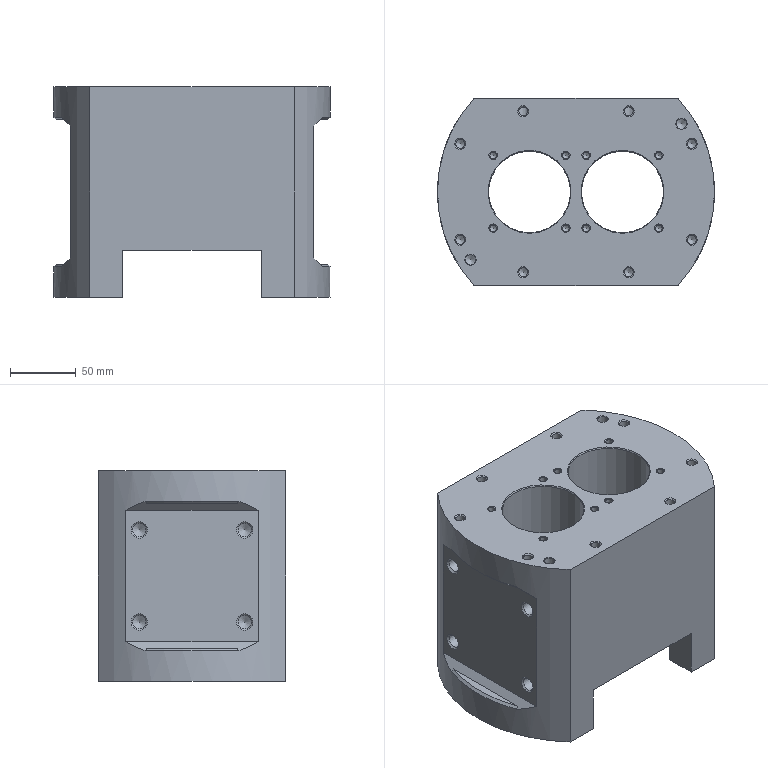NC program | NX | posted with a generic post | part box 210 x 142 x 160 mm
Lines 2120 to 2980 of 4730:
(ZLEVEL_PROFILE_COPY_1 , TOOL : D6R0.5)
N4226 T05 M6
N4228 G54
N4230 G17 G0 G90 X-53.624 Y12.862 B0. C0. S6500 M3
N4232 G43 Z30. H5
N4234 Z2.929
N4236 G94 G1 Z-0.071 F1000.
N4238 X-54.419 Y12.28
N4240 G3 X-54.662 Y11.731 R0.6
N4242 G2 X-54.662 Y-11.732 R108.942 F2500.
N4244 G1 X-54.661 Y-11.887 Z-0.088
N4246 Y-12.042 Z-0.106
N4248 X-54.662 Y-12.197 Z-0.124
N4250 X-54.665 Y-12.351 Z-0.141
N4252 G3 X-54.664 Y12.355 R108.184
N4254 G1 X-54.663 Y12.506 Z-0.159
N4256 Y12.656 Z-0.177
N4258 X-54.664 Y12.806 Z-0.194
N4260 X-54.667 Y12.956 Z-0.212
N4262 G2 X-54.667 Y-12.956 R107.566
N4264 G1 X-54.664 Y-13.103 Z-0.23
N4266 X-54.665 Y-13.25 Z-0.247
N4268 Y-13.397 Z-0.265
N4270 X-54.667 Y-13.544 Z-0.283
N4272 G3 X-54.667 Y13.542 R108.057
N4274 G1 X-54.666 Y13.687 Z-0.301
N4276 X-54.667 Y13.831 Z-0.318
N4278 Y13.976 Z-0.336
N4280 X-54.669 Y14.12 Z-0.354
N4282 G2 X-54.668 Y-14.125 R108.183
N4284 G1 X-54.666 Y-14.262 Z-0.371
N4286 Y-14.399 Z-0.389
N4288 X-54.667 Y-14.536 Z-0.407
N4290 X-54.671 Y-14.673 Z-0.424
N4292 G3 X-54.671 Y14.674 R108.33
N4294 G1 X-54.667 Y14.844 Z-0.448
N4296 X-54.668 Y15.013 Z-0.471
N4298 X-54.671 Y15.183 Z-0.495
N4300 G2 X-54.671 Y-15.18 R108.224
N4302 G1 Y-15.344 Z-0.519
N4304 Y-15.508 Z-0.542
N4306 X-54.674 Y-15.672 Z-0.566
N4308 G3 X-54.674 Y15.674 R107.882
N4310 G1 X-54.672 Y15.835 Z-0.589
N4312 Y15.997 Z-0.613
N4314 X-54.675 Y16.158 Z-0.636
N4316 G2 X-54.675 Y-16.159 R107.945
N4318 G1 X-54.673 Y-16.318 Z-0.66
N4320 X-54.674 Y-16.476 Z-0.684
N4322 X-54.675 Y-16.635 Z-0.707
N4324 G3 X-54.675 Y16.633 R108.072
N4326 G1 Y16.79 Z-0.731
N4328 Y16.946 Z-0.754
N4330 X-54.679 Y17.103 Z-0.778
N4332 G2 X-54.678 Y-17.107 R108.254
N4334 G1 X-54.675 Y-17.257 Z-0.801
N4336 X-54.676 Y-17.407 Z-0.825
N4338 X-54.679 Y-17.556 Z-0.849
N4340 G3 X-54.679 Y17.557 R108.475
N4342 G1 X-54.677 Y17.702 Z-0.872
N4344 Y17.846 Z-0.896
N4346 X-54.679 Y17.99 Z-0.919
N4348 G2 X-54.679 Y-17.988 R108.62
N4350 G1 X-54.68 Y-18.126 Z-0.943
N4352 Y-18.264 Z-0.966
N4354 X-54.682 Y-18.402 Z-0.99
N4356 G3 X-54.682 Y18.404 R108.324
N4358 G1 X-54.681 Y18.541 Z-1.014
N4360 Y18.678 Z-1.037
N4362 X-54.685 Y18.815 Z-1.061
N4364 G2 X-54.685 Y-18.815 R108.248
N4366 G1 X-54.682 Y-18.951 Z-1.084
N4368 X-54.683 Y-19.086 Z-1.108
N4370 X-54.686 Y-19.221 Z-1.131
N4372 G3 X-54.686 Y19.221 R108.276
N4374 G1 X-54.684 Y19.354 Z-1.155
N4376 X-54.685 Y19.487 Z-1.179
N4378 X-54.687 Y19.62 Z-1.202
N4380 G2 X-54.687 Y-19.622 R108.378
N4382 G1 X-54.685 Y-19.756 Z-1.226
N4384 Y-19.889 Z-1.249
N4386 X-54.687 Y-20.022 Z-1.273
N4388 G3 X-54.688 Y20.019 R108.63
N4390 G1 X-54.687 Y20.147 Z-1.296
N4392 Y20.274 Z-1.32
N4394 X-54.688 Y20.401 Z-1.344
N4396 G2 X-54.688 Y-20.401 R108.747
N4398 G1 Y-20.526 Z-1.367
N4400 Y-20.65 Z-1.391
N4402 X-54.69 Y-20.775 Z-1.414
N4404 G3 X-54.689 Y20.778 R108.773
N4406 G1 Y20.897 Z-1.438
N4408 X-54.69 Y21.016 Z-1.461
N4410 X-54.691 Y21.135 Z-1.485
N4412 G2 X-54.691 Y-21.132 R108.599
N4414 G1 Y-21.251 Z-1.508
N4416 X-54.692 Y-21.37 Z-1.532
N4418 X-54.693 Y-21.489 Z-1.556
N4420 G3 X-54.693 Y21.49 R108.585
N4422 G1 X-54.692 Y21.608 Z-1.579
N4424 X-54.693 Y21.726 Z-1.603
N4426 X-54.695 Y21.844 Z-1.626
N4428 G2 X-54.695 Y-21.844 R108.601
N4430 G1 X-54.694 Y-22.017 Z-1.662
N4432 X-54.695 Y-22.189 Z-1.697
N4434 G3 X-54.695 Y22.188 R108.586
N4436 G1 Y22.36 Z-1.732
N4438 X-54.696 Y22.531 Z-1.768
N4440 G2 X-52.49 Y-5.881 R108.93
N4442 X-54.696 Y-22.532 R111.727
N4444 G1 X-54.695 Y-22.703 Z-1.803
N4446 X-54.696 Y-22.874 Z-1.838
N4448 G3 X-52.291 Y-2.768 R111.416
N4450 X-54.697 Y22.872 R109.773
N4452 G1 X-54.696 Y23.036 Z-1.874
N4454 X-54.697 Y23.2 Z-1.909
N4456 G2 X-52.22 Y-2.768 R110.042
N4458 X-54.697 Y-23.2 R111.413
N4460 G1 Y-23.362 Z-1.945
N4462 X-54.698 Y-23.524 Z-1.98
N4464 G3 X-52.152 Y2.768 R109.879
N4466 X-54.697 Y23.525 R111.361
N4468 G1 X-54.696 Y23.683 Z-2.015
N4470 X-54.698 Y23.84 Z-2.051
N4472 G2 X-52.188 Y5.535 R112.247
N4474 X-52.188 Y-5.535 R122.471
N4476 X-54.699 Y-23.838 R112.088
N4478 G1 Y-23.992 Z-2.086
N4480 X-54.7 Y-24.146 Z-2.122
N4482 G3 X-52.121 Y-5.535 R111.188
N4484 X-52.121 Y5.535 R171.637
N4486 X-54.7 Y24.148 R111.301
N4488 G1 X-54.699 Y24.302 Z-2.157
N4490 X-54.702 Y24.454 Z-2.192
N4492 G2 X-52.227 Y8.302 R112.524
N4494 G1 X-52.084 Y5.881
N4496 X-52.07 Y5.535
N4498 G2 X-52.07 Y-5.535 R256.64
N4500 X-53.483 Y-18.335 R102.084
N4502 X-54.702 Y-24.454 R104.38
N4504 G1 X-54.7 Y-24.609 Z-2.228
N4506 X-54.703 Y-24.762 Z-2.263
N4508 G3 X-52.28 Y-9.779 R111.73
N4510 X-52.023 Y-4.713 R60.658
N4512 X-52.023 Y4.713 R498.143
N4514 X-52.159 Y8.302 R64.784
N4516 X-54.703 Y24.762 R111.682
N4518 G1 X-54.701 Y24.916 Z-2.299
N4520 X-54.704 Y25.069 Z-2.334
N4522 G2 X-52.097 Y8.302 R109.91
N4524 X-52. Y3.91 R99.303
N4526 G1 Y-3.91
N4528 G2 X-52.097 Y-8.302 R99.276
N4530 X-54.704 Y-25.071 R109.974
N4532 G1 X-54.702 Y-25.225 Z-2.37
N4534 X-54.705 Y-25.379 Z-2.405
N4536 G3 X-53.78 Y-21.102 R105.979
N4538 X-52.092 Y-8.994 R103.636
N4540 X-52. Y-5.554 R64.677
N4542 G1 Y4.497
N4544 G3 X-52.056 Y8.302 R101.781
N4546 X-52.268 Y11.07 R50.215
N4548 X-54.705 Y25.377 R113.821
N4550 G1 X-54.703 Y25.53 Z-2.441
N4552 X-54.706 Y25.682 Z-2.477
N4554 G2 X-52.203 Y11.127 R114.462
N4556 X-52.021 Y8.053 R33.214
N4558 G1 X-52.002 Y6.573
N4560 X-52.001 Y6.227
N4562 X-52. Y6.034
N4564 Y-6.043
N4566 X-52.002 Y-6.573
N4568 X-52.021 Y-8.033
N4570 G2 X-52.208 Y-11.166 R33.626
N4572 X-54.705 Y-25.684 R115.067
N4574 G1 X-54.704 Y-25.832 Z-2.512
N4576 X-54.706 Y-25.979 Z-2.548
N4578 G3 X-52.132 Y-11.07 R113.634
N4580 X-52. Y-7.145 R49.439
N4582 G1 Y7.148
N4584 G3 X-52.132 Y11.07 R49.422
N4586 X-54.706 Y25.978 R113.527
N4588 G1 Y26.125 Z-2.583
N4590 X-54.707 Y26.271 Z-2.619
N4592 G2 X-52.104 Y11.416 R111.997
N4594 X-52. Y8.105 R46.027
N4596 G1 Y-8.107
N4598 G2 X-52.104 Y-11.416 R46.02
N4600 X-54.707 Y-26.271 R111.928
N4602 G1 Y-26.415 Z-2.654
N4604 X-54.709 Y-26.56 Z-2.69
N4606 G3 X-52.31 Y-13.837 R115.903
N4608 G1 X-52.203 Y-12.938
N4610 G3 X-52. Y-9.511 R28.979
N4612 G1 Y9.511
N4614 G3 X-52.203 Y12.938 R28.98
N4616 G1 X-52.31 Y13.837
N4618 G3 X-54.709 Y26.562 R116.198
N4620 G1 X-54.708 Y26.702 Z-2.726
N4622 X-54.711 Y26.842 Z-2.761
N4624 G2 X-52.273 Y14.101 R116.39
N4626 X-52. Y10.008 R30.803
N4628 G1 Y-10.002
N4630 G2 X-52.274 Y-14.106 R30.884
N4632 X-54.711 Y-26.84 R116.146
N4634 G1 X-54.71 Y-26.979 Z-2.797
N4636 X-54.712 Y-27.117 Z-2.833
N4638 G3 X-52.279 Y-14.701 R116.024
N4640 X-52. Y-10.474 R29.016
N4642 G1 Y10.472
N4644 G3 X-52.171 Y13.837 R29.025
N4646 X-54.712 Y27.118 R114.844
N4648 G1 X-54.711 Y27.257 Z-2.868
N4650 X-54.713 Y27.395 Z-2.904
N4652 G2 X-52.149 Y14.183 R113.767
N4654 X-52. Y11.151 R27.317
N4656 G1 Y-11.149
N4658 G2 X-52.149 Y-14.183 R27.331
N4660 X-54.713 Y-27.395 R113.711
N4662 G1 X-54.712 Y-27.534 Z-2.94
N4664 X-54.713 Y-27.672 Z-2.975
N4666 G3 X-52.211 Y-15.134 R113.722
N4668 X-52. Y-12.135 R21.39
N4670 G1 Y12.135
N4672 G3 X-52.211 Y15.135 R21.395
N4674 X-54.713 Y27.672 R113.682
N4676 G1 X-54.714 Y27.811 Z-3.011
N4678 X-54.716 Y27.949 Z-3.047
N4680 G2 X-52.354 Y16.605 R116.391
N4682 G1 X-52.211 Y15.622
N4684 G2 X-52. Y12.696 R20.357
N4686 G1 Y-12.696
N4688 G2 X-52.211 Y-15.622 R20.357
N4690 X-54.715 Y-27.95 R112.004
N4692 G1 Y-28.09 Z-3.083
N4694 X-54.718 Y-28.228 Z-3.118
N4696 G3 X-52.284 Y-16.605 R117.125
N4698 X-52. Y-12.973 R21.452
N4700 G1 Y12.969
N4702 G3 X-52.284 Y16.605 R21.459
N4704 X-54.718 Y28.226 R116.838
N4706 G1 X-54.716 Y28.363 Z-3.154
N4708 X-54.719 Y28.499 Z-3.19
N4710 G2 X-52.266 Y16.951 R118.709
N4712 X-52. Y13.525 R20.32
N4714 G1 Y-13.521
N4716 G2 X-52.266 Y-16.951 R20.324
N4718 X-54.718 Y-28.501 R119.038
N4720 G1 X-54.717 Y-28.635 Z-3.226
N4722 X-54.719 Y-28.767 Z-3.262
N4724 G3 X-52.265 Y-17.403 R120.193
N4726 X-52. Y-14.053 R19.739
N4728 G1 Y14.053
N4730 G3 X-52.196 Y16.951 R19.737
N4732 X-54.719 Y28.766 R119.041
N4734 G1 Y28.899 Z-3.297
N4736 X-54.72 Y29.031 Z-3.333
N4738 G2 X-52.186 Y17.297 R117.377
N4740 X-52.003 Y14.875 R16.206
N4742 G1 X-52. Y14.529
N4744 Y-14.529
N4746 X-52.003 Y-14.875
N4748 G2 X-52.219 Y-17.506 R16.206
N4750 X-54.72 Y-29.031 R117.118
N4752 G1 X-54.721 Y-29.163 Z-3.369
N4754 X-54.723 Y-29.294 Z-3.405
N4756 G3 X-52.125 Y-17.297 R112.998
N4758 X-52. Y-15.057 R18.234
N4760 G1 Y15.062
N4762 G3 X-52.125 Y17.297 R18.22
N4764 X-54.723 Y29.296 R113.229
N4766 G1 X-54.721 Y29.425 Z-3.441
N4768 X-54.724 Y29.554 Z-3.477
N4770 G2 X-52.222 Y18.335 R116.398
N4772 X-52. Y15.536 R15.623
N4774 G1 Y-15.539
N4776 G2 X-52.222 Y-18.335 R15.621
N4778 X-54.724 Y-29.552 R116.163
N4780 G1 X-54.723 Y-29.679 Z-3.513
N4782 X-54.725 Y-29.805 Z-3.549
N4784 G3 X-52.268 Y-19.038 R119.173
N4786 X-52. Y-16.034 R16.97
N4788 G1 Y16.002
N4790 G3 X-52.21 Y18.681 R15.551
N4792 G1 X-52.329 Y19.372
N4794 G3 X-54.725 Y29.806 R120.037
N4796 G1 Y29.932 Z-3.584
N4798 X-54.726 Y30.058 Z-3.62
N4800 G2 X-52.258 Y19.372 R119.217
N4802 X-52. Y16.453 R15.52
N4804 G1 Y-16.452
N4806 G2 X-52.258 Y-19.372 R15.522
N4808 X-54.726 Y-30.058 R119.039
N4810 G1 Y-30.183 Z-3.656
N4812 X-54.728 Y-30.309 Z-3.692
N4814 G3 X-52.265 Y-19.814 R119.623
N4816 X-52. Y-16.894 R15.45
N4818 G1 Y16.89
N4820 G3 X-52.189 Y19.372 R15.454
N4822 X-54.728 Y30.309 R118.078
N4824 G1 Y30.435 Z-3.728
N4826 X-54.73 Y30.56 Z-3.764
N4828 G2 X-52.182 Y19.718 R118.332
N4830 X-52. Y17.297 R14.774
N4832 G1 Y-17.519
N4834 G2 X-52.228 Y-19.962 R13.223
N4836 X-54.73 Y-30.561 R118.437
N4838 G1 X-54.729 Y-30.687 Z-3.8
N4840 X-54.73 Y-30.814 Z-3.836
N4842 G3 X-52.24 Y-20.395 R118.832
N4844 X-52. Y-17.739 R13.408
N4846 G1 Y17.736
N4848 G3 X-52.18 Y20.064 R13.412
N4850 X-54.73 Y30.813 R117.285
N4852 G1 X-54.731 Y30.939 Z-3.872
N4854 X-54.733 Y31.065 Z-3.908
N4856 G2 X-52.244 Y20.756 R117.486
N4858 X-52. Y18.147 R13.028
N4860 G1 Y-18.144
N4862 G2 X-52.244 Y-20.756 R13.034
N4864 X-54.732 Y-31.066 R117.803
N4866 G1 X-54.731 Y-31.19 Z-3.944
N4868 X-54.734 Y-31.312 Z-3.98
N4870 G3 X-52.241 Y-21.102 R118.205
N4872 X-52. Y-18.545 R12.414
N4874 G1 Y18.543
N4876 G3 X-52.241 Y21.102 R12.417
N4878 X-54.734 Y31.311 R117.909
N4880 G1 X-54.733 Y31.433 Z-4.016
N4882 X-54.735 Y31.554 Z-4.052
N4884 G2 X-52.239 Y21.448 R119.022
N4886 X-52. Y18.936 R12.33
N4888 G1 Y-18.934
N4890 G2 X-52.239 Y-21.448 R12.333
N4892 X-54.735 Y-31.556 R119.233
N4894 G1 Y-31.676 Z-4.089
N4896 X-54.737 Y-31.797 Z-4.125
N4898 G3 X-52.269 Y-21.965 R123.339
N4900 X-52. Y-19.353 R12.843
N4902 G1 Y19.353
N4904 G3 X-52.268 Y21.965 R12.842
N4906 X-54.737 Y31.796 R123.305
N4908 G1 Y31.917 Z-4.161
N4910 X-54.739 Y32.038 Z-4.197
N4912 G2 X-52.27 Y22.32 R124.201
N4914 X-52. Y19.734 R12.498
N4916 G1 Y-19.733
N4918 G2 X-52.27 Y-22.32 R12.506
N4920 X-54.739 Y-32.037 R124.017
N4922 G1 X-54.738 Y-32.157 Z-4.233
N4924 X-54.74 Y-32.276 Z-4.269
N4926 G3 X-52.235 Y-22.486 R124.398
N4928 X-52. Y-20.064 R11.8
N4930 G1 Y20.061
N4932 G3 X-52.235 Y22.486 R11.803
N4934 X-54.74 Y32.277 R124.732
N4936 G1 X-54.739 Y32.395 Z-4.305
N4938 X-54.741 Y32.513 Z-4.342
N4940 G2 X-52.171 Y22.486 R121.069
N4942 X-52. Y20.41 R11.593
N4944 G1 Y-20.41
N4946 G2 X-52.265 Y-22.965 R11.593
N4948 X-54.741 Y-32.512 R124.917
N4950 G1 X-54.742 Y-32.628 Z-4.378
N4952 X-54.744 Y-32.744 Z-4.414
N4954 G3 X-52.249 Y-23.178 R119.251
N4956 X-52. Y-20.756 R10.64
N4958 G1 Y20.756
N4960 G3 X-52.249 Y23.178 R10.64
N4962 X-54.744 Y32.744 R119.355
N4964 G1 Y32.86 Z-4.45
N4966 X-54.745 Y32.976 Z-4.487
N4968 G2 X-52.256 Y23.524 R118.507
N4970 X-52. Y21.102 R10.292
N4972 G1 Y-21.102
N4974 G2 X-52.256 Y-23.524 R10.292
N4976 X-54.745 Y-32.976 R118.515
N4978 G1 Y-33.092 Z-4.523
N4980 X-54.746 Y-33.208 Z-4.559
N4982 G3 X-52.263 Y-23.87 R119.264
N4984 X-52. Y-21.475 R10.213
N4986 G1 Y21.473
N4988 G3 X-52.263 Y23.87 R10.215
N4990 X-54.746 Y33.207 R119.015
N4992 G1 X-54.747 Y33.323 Z-4.595
N4994 X-54.749 Y33.439 Z-4.632
N4996 G2 X-52.269 Y24.216 R119.882
N4998 X-52. Y21.813 R10.236
N5000 G1 Y-21.812
N5002 G2 X-52.269 Y-24.216 R10.237
N5004 X-54.749 Y-33.44 R120.244
N5006 G1 Y-33.557 Z-4.668
N5008 X-54.75 Y-33.673 Z-4.704
N5010 G3 X-52.283 Y-24.607 R126.618
N5012 X-52. Y-22.146 R10.859
N5014 G1 Y22.147
N5016 G3 X-52.281 Y24.601 R10.842
N5018 X-54.751 Y33.671 R125.317
N5020 G1 Y33.787 Z-4.741
N5022 X-54.752 Y33.904 Z-4.777
N5024 G2 X-52.282 Y24.907 R127.556
N5026 X-52. Y22.474 R10.327
N5028 G1 Y-22.475
N5030 G2 X-52.282 Y-24.907 R10.327
N5032 X-54.752 Y-33.906 R128.657
N5034 G1 Y-34.02 Z-4.813
N5036 X-54.753 Y-34.134 Z-4.85
N5038 G3 X-52.267 Y-25.139 R129.086
N5040 X-52. Y-22.864 R9.829
N5042 G1 Y22.8
N5044 G3 X-52.212 Y24.907 R10.382
N5046 X-54.754 Y34.131 R127.264
N5048 G1 Y34.244 Z-4.886
N5050 X-54.756 Y34.357 Z-4.922
N5052 G2 X-52.26 Y25.388 R124.803
N5054 X-52. Y23.18 R9.519
N5056 G1 Y-23.119
N5058 G2 X-52.275 Y-25.48 R9.798
N5060 X-54.754 Y-34.363 R133.924
N5062 G1 Y-34.477 Z-4.959
N5064 X-54.755 Y-34.591 Z-4.995
N5066 G3 X-52.367 Y-26.119 R129.855
N5068 G1 X-52.239 Y-25.599
N5070 X-52.163 Y-25.253
N5072 G3 X-52. Y-23.431 R9.614
N5074 G1 Y23.432
N5076 G3 X-52.163 Y25.253 R9.612
N5078 G1 X-52.239 Y25.599
N5080 X-52.367 Y26.119
N5082 G3 X-54.757 Y34.584 R125.401
N5084 G1 X-54.758 Y34.697 Z-5.032
N5086 X-54.759 Y34.81 Z-5.068
N5088 G2 X-52.255 Y25.945 R127.029
N5090 X-52. Y23.742 R8.98
N5092 G1 Y-23.742
N5094 G2 X-52.255 Y-25.945 R8.98
N5096 X-54.757 Y-34.819 R131.3
N5098 G1 X-54.751 Y-34.917 Z-5.105
N5100 X-54.746 Y-35.014 Z-5.141
N5102 G3 X-52.262 Y-26.263 R137.055
N5104 X-52. Y-24.118 R8.899
N5106 G1 Y24.048
N5108 G3 X-52.27 Y26.291 R8.683
N5110 X-54.749 Y35.008 R129.719
N5112 G1 X-54.725 Y35.168 Z-5.214
N5114 G2 X-52.274 Y26.599 R141.147
N5116 X-52. Y24.391 R9.028
N5118 G1 Y-24.399
N5120 G2 X-52.261 Y-26.541 R8.919
N5122 X-54.095 Y-33.13 R117.669
N5124 G1 X-54.656 Y-34.94
N5126 X-54.722 Y-35.174
N5128 X-54.691 Y-35.32 Z-5.287
N5130 X-54.433 Y-34.434
N5132 G3 X-52.281 Y-26.914 R127.907
N5134 X-52. Y-24.658 R9.187
N5136 G1 Y24.67
N5138 G3 X-52.277 Y26.896 R9.089
N5140 X-53.943 Y32.864 R125.038
N5142 G1 X-54.048 Y33.21
N5144 X-54.589 Y34.94
N5146 X-54.693 Y35.316
N5148 X-54.646 Y35.433 Z-5.36
N5150 X-54.614 Y35.286
N5152 X-54.304 Y34.248
N5154 X-54.194 Y33.902
N5156 G2 X-52.293 Y27.252 R135.702
N5158 X-52. Y24.949 R9.2
N5160 G1 Y-24.949
N5162 G2 X-52.293 Y-27.252 R9.199
N5164 X-54.413 Y-34.594 R135.255
N5166 G1 X-54.611 Y-35.286
N5168 X-54.645 Y-35.435
N5170 X-54.585 Y-35.554 Z-5.433
N5172 G2 X-54.416 Y-34.819 R4.415
N5174 G3 X-52.289 Y-27.509 R135.481
N5176 X-52. Y-25.255 R8.934
N5178 G1 Y25.254
N5180 G3 X-52.29 Y27.513 R8.937
N5182 X-54.43 Y34.869 R138.234
N5184 G2 X-54.585 Y35.554 R3.93
N5186 G1 X-54.516 Y35.677 Z-5.506
N5188 G3 X-54.38 Y34.94 R2.795
N5190 G2 X-52.29 Y27.782 R148.3
N5192 X-52. Y25.557 R8.685
N5194 G1 Y-25.557
N5196 G2 X-52.288 Y-27.776 R8.685
N5198 X-54.383 Y-34.94 R142.479
N5200 G3 X-54.517 Y-35.675 R3.009
N5202 G1 X-54.449 Y-35.803 Z-5.577
N5204 G2 X-54.316 Y-34.94 R3.033
N5206 G3 X-52.275 Y-27.979 R137.677
N5208 X-52. Y-25.869 R8.241
N5210 G1 Y25.865
N5212 G3 X-52.275 Y27.982 R8.279
N5214 X-53.987 Y33.902 R135.073
N5216 G1 X-54.207 Y34.594
N5218 X-54.312 Y34.94
N5220 G2 X-54.446 Y35.805 R2.77
N5222 G1 X-54.374 Y35.926 Z-5.649
N5224 X-54.339 Y35.286
N5226 X-54.244 Y34.94
N5228 X-53.604 Y32.873
N5230 G2 X-52.254 Y28.143 R109.145
N5232 X-52. Y26.167 R7.819
N5234 G1 Y-26.159
N5236 G2 X-52.263 Y-28.182 R7.913
N5238 X-54.222 Y-34.85 R127.872
N5240 G3 X-54.378 Y-35.924 R3.225
N5242 G1 X-54.311 Y-36.051 Z-5.72
N5244 X-54.271 Y-35.286
N5246 G2 X-54.038 Y-34.487 R15.81
N5248 G3 X-52.244 Y-28.367 R125.478
N5250 X-52. Y-26.351 R7.792
N5252 G1 Y26.425
N5254 G3 X-52.291 Y28.549 R7.903
N5256 G1 X-53.012 Y31.134
N5258 X-53.115 Y31.48
N5260 X-54.177 Y34.94
N5262 X-54.274 Y35.286
N5264 X-54.308 Y36.055
N5266 X-54.241 Y36.191 Z-5.791
N5268 X-54.209 Y35.286
N5270 X-52.945 Y31.134
N5272 X-52.843 Y30.788
N5274 X-52.27 Y28.713
N5276 X-52.181 Y28.367
N5278 G2 X-52. Y26.619 R7.907
N5280 G1 Y-26.616
N5282 G2 X-52.27 Y-28.713 R7.669
N5284 X-54.039 Y-34.699 R123.041
N5286 G3 X-54.205 Y-35.286 R8.465
N5288 G1 X-54.246 Y-36.186
N5290 X-54.177 Y-36.321 Z-5.862
N5292 X-54.139 Y-35.286
N5294 G2 X-53.968 Y-34.69 R9.028
N5296 G3 X-52.264 Y-28.939 R122.605
N5298 X-52. Y-26.947 R7.644
N5300 G1 Y26.949
N5302 G3 X-52.28 Y29.003 R7.687
N5304 G1 X-52.775 Y30.788
N5306 X-52.877 Y31.134
N5308 X-54.144 Y35.286
N5310 X-54.172 Y36.328
N5312 X-54.137 Y36.422 Z-5.898
N5314 X-54.105 Y36.517 Z-5.933
N5316 X-54.102 Y36.323
N5318 X-54.08 Y35.459
N5320 Y35.286
N5322 G2 X-52.287 Y29.278 R170.492
N5324 X-52. Y27.18 R7.82
N5326 G1 Y-27.186
N5328 G2 X-52.272 Y-29.217 R7.725
N5330 X-53.915 Y-34.731 R121.979
N5332 G3 X-54.072 Y-35.286 R7.806
N5334 G1 X-54.106 Y-36.323
N5336 X-54.109 Y-36.512
N5338 X-54.072 Y-36.607 Z-5.969
N5340 X-54.038 Y-36.703 Z-6.004
N5342 X-54.006 Y-35.317
N5344 G2 X-53.971 Y-35.112 R0.713
N5346 G3 X-52.279 Y-29.496 R126.921
N5348 X-52. Y-27.436 R7.739
N5350 G1 Y27.432
N5352 G3 X-52.287 Y29.526 R7.788
N5354 X-54.02 Y35.286 R150.329
N5356 G1 X-54.035 Y36.707
N5358 X-53.999 Y36.802 Z-6.039
N5360 X-53.969 Y36.896 Z-6.075
N5362 X-53.959 Y35.286
N5364 G2 X-52.287 Y29.776 R137.348
N5366 X-52. Y27.69 R7.719
N5368 G1 Y-27.691
N5370 G2 X-52.286 Y-29.769 R7.706
N5372 X-53.895 Y-35.085 R132.105
N5374 G3 X-53.942 Y-35.359 R0.941
N5376 G1 X-53.971 Y-36.894
N5378 X-53.932 Y-36.989 Z-6.11
N5380 X-53.899 Y-37.084 Z-6.145
N5382 X-53.877 Y-35.286
N5384 X-53.67 Y-34.594
N5386 G3 X-52.303 Y-30.081 R143.933
N5388 X-52. Y-27.915 R7.898
N5390 G1 Y27.912
N5392 G3 X-52.304 Y30.084 R7.922
N5394 X-53.894 Y35.286 R143.061
N5396 G1 X-53.898 Y37.085
N5398 X-53.861 Y37.179 Z-6.181
N5400 X-53.829 Y37.273 Z-6.216
N5402 X-53.82 Y35.632
N5404 X-53.826 Y35.286
N5406 G2 X-52.337 Y30.442 R151.821
N5408 X-52. Y28.16 R7.827
N5410 G1 Y-28.159
N5412 G2 X-52.337 Y-30.442 R7.827
N5414 X-53.816 Y-35.285 R237.605
N5416 G1 X-53.829 Y-37.272
N5418 X-53.791 Y-37.365 Z-6.251
N5420 X-53.759 Y-37.459 Z-6.287
N5422 X-53.753 Y-35.977
N5424 X-53.751 Y-35.377
N5426 X-53.756 Y-35.325
N5428 Y-35.271
N5430 G3 X-52.294 Y-30.525 R144.779
N5432 X-52. Y-28.453 R7.453
N5434 G1 Y28.453
N5436 G3 X-52.294 Y30.524 R7.453
N5438 X-53.756 Y35.271 R144.281
N5440 G1 Y35.38
N5442 X-53.755 Y35.632
N5444 X-53.756 Y37.361
N5446 X-53.758 Y37.459
N5448 X-53.72 Y37.552 Z-6.322
N5450 X-53.686 Y37.645 Z-6.357
N5452 X-53.685 Y35.576
N5454 Y35.266
N5456 G2 X-52.287 Y30.729 R149.74
N5458 X-52. Y28.713 R7.217
N5460 G1 Y-28.713
N5462 G2 X-52.287 Y-30.729 R7.216
N5464 X-53.685 Y-35.266 R149.74
N5466 G1 Y-35.541
N5468 X-53.68 Y-35.585
N5470 X-53.687 Y-37.644
N5472 X-53.65 Y-37.737 Z-6.393
N5474 X-53.62 Y-37.829 Z-6.428
N5476 X-53.615 Y-35.773
N5478 Y-35.254
N5480 G3 X-52.277 Y-30.918 R140.432
N5482 X-52. Y-28.972 R6.967
N5484 G1 Y28.972
N5486 G3 X-52.277 Y30.918 R6.967
N5488 X-53.615 Y35.254 R140.432
N5490 G1 Y35.773
N5492 X-53.614 Y37.707
N5494 X-53.619 Y37.83
N5496 X-53.579 Y37.922 Z-6.464
N5498 X-53.546 Y38.015 Z-6.499
N5500 X-53.544 Y37.707
N5502 Y35.967
N5504 Y35.242
N5506 G2 X-52.275 Y31.134 R128.258
N5508 X-52. Y29.137 R6.756
N5510 G1 Y-29.137
N5512 G2 X-52.275 Y-31.134 R6.758
N5514 X-53.544 Y-35.242 R128.258
N5516 G1 X-53.543 Y-35.977
N5518 X-53.546 Y-38.014
N5520 X-53.509 Y-38.107 Z-6.534
N5522 X-53.477 Y-38.2 Z-6.57
N5524 X-53.473 Y-38.053
N5526 X-53.472 Y-36.323
N5528 X-53.473 Y-36.16
N5530 Y-35.23
N5532 G3 X-52.271 Y-31.345 R120.873
N5534 X-52. Y-29.448 R6.786
N5536 G1 Y29.448
N5538 G3 X-52.27 Y31.344 R6.785
N5540 X-53.473 Y35.23 R120.479
N5542 G1 Y36.16
N5544 X-53.472 Y36.323
N5546 X-53.473 Y38.053
N5548 X-53.477 Y38.2
N5550 X-53.438 Y38.293 Z-6.605
N5552 X-53.403 Y38.386 Z-6.64
N5554 Y36.352
N5556 Y35.218
N5558 G2 X-52.245 Y31.48 R112.41
N5560 X-52. Y29.615 R6.807
N5562 G1 Y-29.614
N5564 G2 X-52.245 Y-31.48 R6.807
N5566 X-53.403 Y-35.218 R112.41
N5568 G1 Y-36.352
N5570 Y-38.385
N5572 X-53.367 Y-38.476 Z-6.676
N5574 X-53.335 Y-38.567 Z-6.711
N5576 X-53.332 Y-38.399
N5578 Y-36.542
N5580 Y-35.206
N5582 G3 X-52.281 Y-31.826 R107.018
N5584 X-52. Y-29.848 R6.637
N5586 G1 Y29.848
N5588 G3 X-52.281 Y31.826 R6.636
N5590 X-53.332 Y35.206 R109.861
N5592 G1 Y36.543
N5594 Y38.399
N5596 X-53.335 Y38.567
N5598 X-53.296 Y38.658 Z-6.746
N5600 X-53.261 Y38.748 Z-6.782
N5602 Y36.734
N5604 Y35.193
N5606 X-52.522 Y32.864
N5608 X-52.29 Y32.089
N5610 G2 X-52. Y30.11 R6.9
N5612 G1 Y-30.11
N5614 G2 X-52.29 Y-32.089 R6.9
N5616 G1 X-52.522 Y-32.864
N5618 X-53.261 Y-35.193
N5620 Y-36.734
N5622 Y-38.748
N5624 X-53.226 Y-38.837 Z-6.817
N5626 X-53.194 Y-38.926 Z-6.852
N5628 X-53.19 Y-38.745
N5630 X-53.189 Y-37.015
N5632 X-53.19 Y-36.669
N5634 Y-35.181
N5636 X-53.115 Y-34.94
N5638 X-52.367 Y-32.573
N5640 G3 X-52. Y-30.314 R7.121
N5642 G1 Y30.319
N5644 G3 X-52.327 Y32.446 R7.067
N5646 G1 X-53.19 Y35.181
N5648 Y36.669
N5650 X-53.189 Y36.925
N5652 X-53.19 Y38.745
N5654 X-53.194 Y38.926
N5656 X-53.155 Y39.015 Z-6.888
N5658 X-53.12 Y39.104 Z-6.923
N5660 X-53.118 Y37.112
N5662 X-53.12 Y37.015
N5664 X-53.119 Y35.159
N5666 X-52.492 Y33.21
N5668 X-52.289 Y32.535
N5670 G2 X-52. Y30.579 R6.775
N5672 G1 Y-30.579
N5674 G2 X-52.289 Y-32.535 R6.775
N5676 G1 X-52.492 Y-33.21
N5678 X-53.119 Y-35.159
N5680 X-53.12 Y-37.015
N5682 X-53.118 Y-37.112
N5684 X-53.12 Y-39.104
N5686 X-53.084 Y-39.193 Z-6.959
N5688 X-53.051 Y-39.282 Z-6.994
N5690 X-53.049 Y-39.091
N5692 X-53.047 Y-37.361
N5694 X-53.049 Y-37.015
N5696 Y-35.146
N5698 X-52.425 Y-33.21
N5700 X-52.295 Y-32.78
N5702 G3 X-52. Y-30.782 R6.915
N5704 G1 Y30.782
N5706 G3 X-52.295 Y32.781 R6.916
N5708 G1 X-52.425 Y33.21
N5710 X-53.049 Y35.146
N5712 Y37.015
N5714 X-53.047 Y37.361
N5716 X-53.049 Y39.091
N5718 X-53.051 Y39.282
N5720 X-53.014 Y39.371 Z-7.029
N5722 X-52.98 Y39.46 Z-7.065
N5724 X-52.978 Y37.361
N5726 Y35.134
N5728 X-52.358 Y33.21
N5730 G2 X-52. Y30.996 R6.998
N5732 G1 Y-30.994
N5734 G2 X-52.358 Y-33.21 R6.998
N5736 G1 X-52.978 Y-35.134
N5738 Y-37.361
N5740 X-52.98 Y-39.46
N5742 X-52.943 Y-39.549 Z-7.1
N5744 X-52.913 Y-39.638 Z-7.135
N5746 X-52.908 Y-39.437
N5748 Y-37.361
N5750 Y-35.131
N5752 X-52.294 Y-33.21
N5754 X-52.264 Y-33.109
N5756 G3 X-52. Y-31.272 R6.522
N5758 G1 Y31.272
N5760 G3 X-52.264 Y33.109 R6.522
N5762 G1 X-52.294 Y33.21
N5764 X-52.908 Y35.131
N5766 Y37.361
N5768 Y39.437
N5770 X-52.913 Y39.638
N5772 X-52.872 Y39.727 Z-7.171
N5774 X-52.838 Y39.815 Z-7.206
N5776 X-52.837 Y39.783
N5778 X-52.836 Y37.852
N5780 X-52.837 Y37.707
N5782 X-52.836 Y35.109
N5784 X-52.318 Y33.503
N5786 G2 X-52. Y31.484 R6.57
N5788 G1 Y-31.484
N5790 G2 X-52.318 Y-33.502 R6.57
N5792 G1 X-52.836 Y-35.109
N5794 X-52.837 Y-37.707
N5796 X-52.836 Y-37.852
N5798 X-52.837 Y-39.783
N5800 X-52.838 Y-39.815
N5802 X-52.802 Y-39.902 Z-7.241
N5804 X-52.77 Y-39.989 Z-7.277
N5806 X-52.766 Y-39.783
N5808 Y-38.032
N5810 Y-35.106
N5812 X-52.272 Y-33.556
N5814 X-52.238 Y-33.434
N5816 G3 X-52. Y-31.737 R6.176
N5818 G1 Y31.737
N5820 G3 X-52.238 Y33.434 R6.176
N5822 G1 X-52.272 Y33.556
N5824 X-52.766 Y35.106
N5826 Y38.033
N5828 Y39.783
N5830 X-52.77 Y39.989
N5832 X-52.731 Y40.076 Z-7.312
N5834 X-52.697 Y40.162 Z-7.347
N5836 X-52.695 Y40.129
N5838 Y38.214
N5840 Y35.083
N5842 X-52.3 Y33.861
N5844 G2 X-52. Y31.954 R6.204
N5846 G1 Y-31.954
N5848 G2 X-52.3 Y-33.861 R6.204
N5850 G1 X-52.695 Y-35.083
N5852 Y-38.214
N5854 Y-40.129
N5856 X-52.697 Y-40.162
N5858 X-52.66 Y-40.248 Z-7.383
N5860 X-52.628 Y-40.333 Z-7.418
N5862 X-52.625 Y-40.129
N5864 X-52.623 Y-38.399
N5866 X-52.625 Y-38.053
N5868 Y-35.081
N5870 X-52.284 Y-34.005
N5872 G3 X-52. Y-32.164 R6.104
N5874 G1 Y32.164
N5876 G3 X-52.284 Y34.005 R6.104
N5878 G1 X-52.625 Y35.081
N5880 Y38.053
N5882 X-52.623 Y38.399
N5884 X-52.625 Y40.129
N5886 X-52.628 Y40.333
N5888 X-52.589 Y40.418 Z-7.453
N5890 X-52.555 Y40.504 Z-7.489
N5892 X-52.552 Y38.576
N5894 X-52.554 Y38.399
N5896 Y35.069
N5898 X-52.265 Y34.142
N5900 G2 X-52. Y32.405 R5.832
N5902 G1 Y-32.405
N5904 G2 X-52.265 Y-34.142 R5.832
N5906 G1 X-52.554 Y-35.069
N5908 Y-38.399
N5910 X-52.552 Y-38.576
N5912 X-52.555 Y-40.504
N5914 X-52.519 Y-40.589 Z-7.524
N5916 X-52.487 Y-40.675 Z-7.56
N5918 X-52.483 Y-40.475
N5920 Y-38.745
N5922 Y-35.046
N5924 X-52.3 Y-34.475
N5926 G3 X-52. Y-32.559 R6.274
N5928 G1 Y32.559
N5930 G3 X-52.3 Y34.475 R6.274
N5932 G1 X-52.483 Y35.046
N5934 Y38.745
N5936 Y40.475
N5938 X-52.487 Y40.675
N5940 X-52.448 Y40.761 Z-7.595